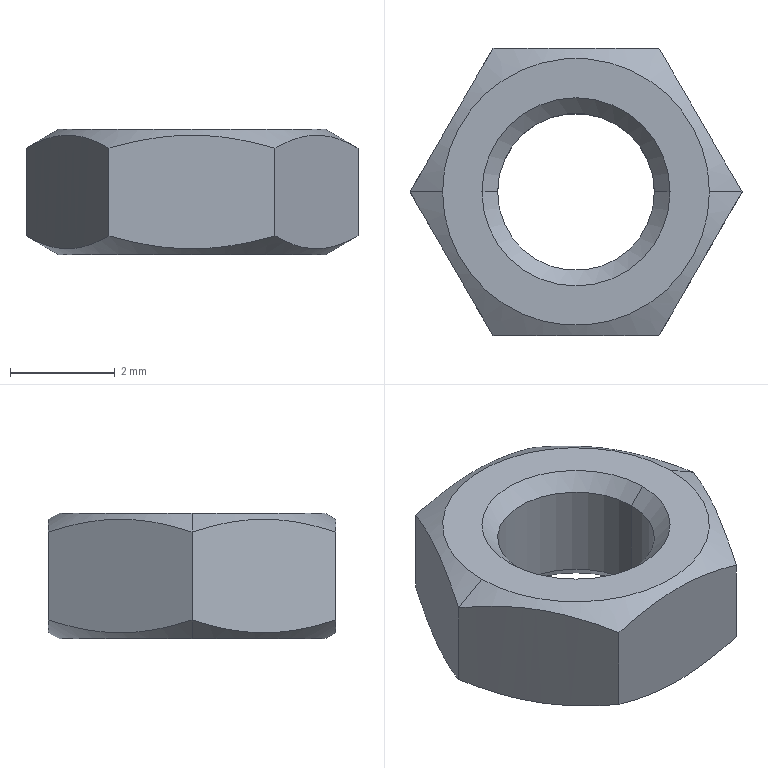Part | SolidWorks | features BaseBody 1 | 1 solid | 18 faces | box 6.351 x 5.5 x 2.4 mm | volume 43.705 mm3 | cone 8 | plane 8 | cylinder 2 | commonest cylinder face diameters 3 x2
STEP:
#1=CARTESIAN_POINT('',(-1.5,0.,2.1));
#2=VERTEX_POINT('',#1);
#3=CARTESIAN_POINT('',(-1.8,0.,2.4));
#4=VERTEX_POINT('',#3);
#5=CARTESIAN_POINT('',(-1.5,0.,2.1));
#6=DIRECTION('',(-0.7071,0.,0.7071));
#7=VECTOR('',#6,1000.);
#8=LINE('',#5,#7);
#9=EDGE_CURVE('',#2,#4,#8,.T.);
#10=ORIENTED_EDGE('',*,*,#9,.F.);
#11=CARTESIAN_POINT('',(1.5,0.,2.1));
#12=VERTEX_POINT('',#11);
#13=CARTESIAN_POINT('',(0.,0.,2.1));
#14=DIRECTION('',(0.,0.,1.));
#15=DIRECTION('',(1.,0.,0.));
#16=AXIS2_PLACEMENT_3D('',#13,#14,#15);
#17=CIRCLE('',#16,1.5);
#18=EDGE_CURVE('',#12,#2,#17,.T.);
#19=ORIENTED_EDGE('',*,*,#18,.F.);
#20=CARTESIAN_POINT('',(1.8,0.,2.4));
#21=VERTEX_POINT('',#20);
#22=CARTESIAN_POINT('',(1.5,0.,2.1));
#23=DIRECTION('',(0.7071,0.,0.7071));
#24=VECTOR('',#23,1000.);
#25=LINE('',#22,#24);
#26=EDGE_CURVE('',#12,#21,#25,.T.);
#27=ORIENTED_EDGE('',*,*,#26,.T.);
#28=CARTESIAN_POINT('',(0.,0.,2.4));
#29=DIRECTION('',(0.,0.,-1.));
#30=DIRECTION('',(1.,0.,0.));
#31=AXIS2_PLACEMENT_3D('',#28,#29,#30);
#32=CIRCLE('',#31,1.8);
#33=EDGE_CURVE('',#4,#21,#32,.T.);
#34=ORIENTED_EDGE('',*,*,#33,.F.);
#35=EDGE_LOOP('',(#10,#19,#27,#34));
#36=FACE_OUTER_BOUND('',#35,.T.);
#37=CARTESIAN_POINT('',(0.,0.,2.1));
#38=DIRECTION('',(0.,0.,1.));
#39=DIRECTION('',(1.,0.,0.));
#40=AXIS2_PLACEMENT_3D('',#37,#38,#39);
#41=CONICAL_SURFACE('',#40,1.5,0.7854);
#42=ADVANCED_FACE('',(#36),#41,.F.);
#43=CARTESIAN_POINT('',(1.5,0.,0.3));
#44=VERTEX_POINT('',#43);
#45=CARTESIAN_POINT('',(1.8,0.,0.));
#46=VERTEX_POINT('',#45);
#47=CARTESIAN_POINT('',(1.8,0.,0.));
#48=DIRECTION('',(0.7071,0.,-0.7071));
#49=VECTOR('',#48,1000.);
#50=LINE('',#47,#49);
#51=EDGE_CURVE('',#44,#46,#50,.T.);
#52=ORIENTED_EDGE('',*,*,#51,.F.);
#53=CARTESIAN_POINT('',(-1.5,0.,0.3));
#54=VERTEX_POINT('',#53);
#55=CARTESIAN_POINT('',(0.,0.,0.3));
#56=DIRECTION('',(0.,0.,-1.));
#57=DIRECTION('',(1.,0.,0.));
#58=AXIS2_PLACEMENT_3D('',#55,#56,#57);
#59=CIRCLE('',#58,1.5);
#60=EDGE_CURVE('',#54,#44,#59,.T.);
#61=ORIENTED_EDGE('',*,*,#60,.F.);
#62=CARTESIAN_POINT('',(-1.8,0.,0.));
#63=VERTEX_POINT('',#62);
#64=CARTESIAN_POINT('',(-1.8,0.,0.));
#65=DIRECTION('',(-0.7071,0.,-0.7071));
#66=VECTOR('',#65,1000.);
#67=LINE('',#64,#66);
#68=EDGE_CURVE('',#54,#63,#67,.T.);
#69=ORIENTED_EDGE('',*,*,#68,.T.);
#70=CARTESIAN_POINT('',(0.,0.,0.));
#71=DIRECTION('',(0.,0.,1.));
#72=DIRECTION('',(1.,0.,0.));
#73=AXIS2_PLACEMENT_3D('',#70,#71,#72);
#74=CIRCLE('',#73,1.8);
#75=EDGE_CURVE('',#46,#63,#74,.T.);
#76=ORIENTED_EDGE('',*,*,#75,.F.);
#77=EDGE_LOOP('',(#52,#61,#69,#76));
#78=FACE_OUTER_BOUND('',#77,.T.);
#79=CARTESIAN_POINT('',(0.,0.,0.));
#80=DIRECTION('',(0.,0.,-1.));
#81=DIRECTION('',(-1.,0.,0.));
#82=AXIS2_PLACEMENT_3D('',#79,#80,#81);
#83=CONICAL_SURFACE('',#82,1.8,0.7854);
#84=ADVANCED_FACE('',(#78),#83,.F.);
#85=CARTESIAN_POINT('',(-2.552,0.,2.4));
#86=VERTEX_POINT('',#85);
#87=CARTESIAN_POINT('',(-3.175,0.,2.04));
#88=VERTEX_POINT('',#87);
#89=CARTESIAN_POINT('',(-2.552,0.,2.4));
#90=DIRECTION('',(-0.866,0.,-0.5));
#91=VECTOR('',#90,1000.);
#92=LINE('',#89,#91);
#93=EDGE_CURVE('',#86,#88,#92,.T.);
#94=ORIENTED_EDGE('',*,*,#93,.F.);
#95=CARTESIAN_POINT('',(2.552,0.,2.4));
#96=VERTEX_POINT('',#95);
#97=CARTESIAN_POINT('',(0.,0.,2.4));
#98=DIRECTION('',(0.,0.,-1.));
#99=DIRECTION('',(-1.,0.,0.));
#100=AXIS2_PLACEMENT_3D('',#97,#98,#99);
#101=CIRCLE('',#100,2.552);
#102=EDGE_CURVE('',#86,#96,#101,.T.);
#103=ORIENTED_EDGE('',*,*,#102,.T.);
#104=CARTESIAN_POINT('',(3.175,0.,2.04));
#105=VERTEX_POINT('',#104);
#106=CARTESIAN_POINT('',(2.552,0.,2.4));
#107=DIRECTION('',(0.866,0.,-0.5));
#108=VECTOR('',#107,1000.);
#109=LINE('',#106,#108);
#110=EDGE_CURVE('',#96,#105,#109,.T.);
#111=ORIENTED_EDGE('',*,*,#110,.T.);
#112=CARTESIAN_POINT('',(1.588,2.75,2.04));
#113=VERTEX_POINT('',#112);
#114=CARTESIAN_POINT('',(3.175,0.,2.04));
#115=CARTESIAN_POINT('',(3.108,0.1168,2.079));
#116=CARTESIAN_POINT('',(3.042,0.2311,2.113));
#117=CARTESIAN_POINT('',(2.944,0.4004,2.158));
#118=CARTESIAN_POINT('',(2.912,0.4564,2.172));
#119=CARTESIAN_POINT('',(2.864,0.5402,2.191));
#120=CARTESIAN_POINT('',(2.848,0.568,2.197));
#121=CARTESIAN_POINT('',(2.816,0.6237,2.208));
#122=CARTESIAN_POINT('',(2.801,0.6497,2.214));
#123=CARTESIAN_POINT('',(2.647,0.9155,2.263));
#124=CARTESIAN_POINT('',(2.518,1.139,2.285));
#125=CARTESIAN_POINT('',(2.316,1.489,2.286));
#126=CARTESIAN_POINT('',(2.249,1.604,2.28));
#127=CARTESIAN_POINT('',(2.149,1.777,2.264));
#128=CARTESIAN_POINT('',(2.116,1.835,2.257));
#129=CARTESIAN_POINT('',(2.066,1.922,2.244));
#130=CARTESIAN_POINT('',(2.049,1.951,2.24));
#131=CARTESIAN_POINT('',(2.015,2.01,2.23));
#132=CARTESIAN_POINT('',(1.997,2.041,2.225));
#133=CARTESIAN_POINT('',(1.852,2.292,2.178));
#134=CARTESIAN_POINT('',(1.723,2.515,2.118));
#135=CARTESIAN_POINT('',(1.588,2.75,2.04));
#136=B_SPLINE_CURVE_WITH_KNOTS('',3,(#114,#115,#116,#117,#118,#119,#120,#121,#122,#123,#124,#125,#126,#127,#128,#129,#130,#131,#132,#133,#134,#135),.UNSPECIFIED.,.F.,.F.,(4,2,2,2,2,2,2,2,2,2,4),(0.,0.125,0.1875,0.2188,0.25,0.5,0.625,0.6875,0.7188,0.75,1.),.UNSPECIFIED.);
#137=EDGE_CURVE('',#105,#113,#136,.T.);
#138=ORIENTED_EDGE('',*,*,#137,.T.);
#139=CARTESIAN_POINT('',(-1.588,2.75,2.04));
#140=VERTEX_POINT('',#139);
#141=CARTESIAN_POINT('',(1.588,2.75,2.04));
#142=CARTESIAN_POINT('',(1.453,2.75,2.079));
#143=CARTESIAN_POINT('',(1.321,2.75,2.113));
#144=CARTESIAN_POINT('',(1.126,2.75,2.158));
#145=CARTESIAN_POINT('',(1.061,2.75,2.172));
#146=CARTESIAN_POINT('',(0.9645,2.75,2.191));
#147=CARTESIAN_POINT('',(0.9324,2.75,2.197));
#148=CARTESIAN_POINT('',(0.8682,2.75,2.208));
#149=CARTESIAN_POINT('',(0.8383,2.75,2.214));
#150=CARTESIAN_POINT('',(0.5302,2.75,2.263));
#151=CARTESIAN_POINT('',(0.2694,2.75,2.286));
#152=CARTESIAN_POINT('',(-0.1341,2.75,2.286));
#153=CARTESIAN_POINT('',(-0.2666,2.75,2.28));
#154=CARTESIAN_POINT('',(-0.4663,2.75,2.263));
#155=CARTESIAN_POINT('',(-0.5331,2.75,2.257));
#156=CARTESIAN_POINT('',(-0.6339,2.75,2.244));
#157=CARTESIAN_POINT('',(-0.6677,2.75,2.24));
#158=CARTESIAN_POINT('',(-0.7355,2.75,2.23));
#159=CARTESIAN_POINT('',(-0.7717,2.75,2.224));
#160=CARTESIAN_POINT('',(-1.06,2.75,2.178));
#161=CARTESIAN_POINT('',(-1.318,2.75,2.118));
#162=CARTESIAN_POINT('',(-1.588,2.75,2.04));
#163=B_SPLINE_CURVE_WITH_KNOTS('',3,(#141,#142,#143,#144,#145,#146,#147,#148,#149,#150,#151,#152,#153,#154,#155,#156,#157,#158,#159,#160,#161,#162),.UNSPECIFIED.,.F.,.F.,(4,2,2,2,2,2,2,2,2,2,4),(0.,0.125,0.1875,0.2187,0.25,0.5,0.625,0.6875,0.7187,0.75,1.),.UNSPECIFIED.);
#164=EDGE_CURVE('',#113,#140,#163,.T.);
#165=ORIENTED_EDGE('',*,*,#164,.T.);
#166=CARTESIAN_POINT('',(-1.588,2.75,2.04));
#167=CARTESIAN_POINT('',(-1.655,2.633,2.079));
#168=CARTESIAN_POINT('',(-1.721,2.519,2.113));
#169=CARTESIAN_POINT('',(-1.819,2.35,2.158));
#170=CARTESIAN_POINT('',(-1.851,2.294,2.172));
#171=CARTESIAN_POINT('',(-1.9,2.21,2.191));
#172=CARTESIAN_POINT('',(-1.916,2.182,2.197));
#173=CARTESIAN_POINT('',(-1.948,2.126,2.208));
#174=CARTESIAN_POINT('',(-1.963,2.1,2.214));
#175=CARTESIAN_POINT('',(-2.116,1.835,2.263));
#176=CARTESIAN_POINT('',(-2.245,1.611,2.285));
#177=CARTESIAN_POINT('',(-2.447,1.261,2.286));
#178=CARTESIAN_POINT('',(-2.514,1.146,2.28));
#179=CARTESIAN_POINT('',(-2.614,0.9728,2.264));
#180=CARTESIAN_POINT('',(-2.647,0.915,2.257));
#181=CARTESIAN_POINT('',(-2.697,0.8278,2.244));
#182=CARTESIAN_POINT('',(-2.714,0.7986,2.24));
#183=CARTESIAN_POINT('',(-2.748,0.7399,2.23));
#184=CARTESIAN_POINT('',(-2.766,0.7087,2.225));
#185=CARTESIAN_POINT('',(-2.911,0.4583,2.178));
#186=CARTESIAN_POINT('',(-3.04,0.2346,2.118));
#187=CARTESIAN_POINT('',(-3.175,0.,2.04));
#188=B_SPLINE_CURVE_WITH_KNOTS('',3,(#166,#167,#168,#169,#170,#171,#172,#173,#174,#175,#176,#177,#178,#179,#180,#181,#182,#183,#184,#185,#186,#187),.UNSPECIFIED.,.F.,.F.,(4,2,2,2,2,2,2,2,2,2,4),(0.,0.125,0.1875,0.2188,0.25,0.5,0.625,0.6875,0.7188,0.75,1.),.UNSPECIFIED.);
#189=EDGE_CURVE('',#140,#88,#188,.T.);
#190=ORIENTED_EDGE('',*,*,#189,.T.);
#191=EDGE_LOOP('',(#94,#103,#111,#138,#165,#190));
#192=FACE_OUTER_BOUND('',#191,.T.);
#193=CARTESIAN_POINT('',(0.,0.,2.4));
#194=DIRECTION('',(0.,0.,-1.));
#195=DIRECTION('',(1.,0.,0.));
#196=AXIS2_PLACEMENT_3D('',#193,#194,#195);
#197=CONICAL_SURFACE('',#196,2.552,1.047);
#198=ADVANCED_FACE('',(#192),#197,.T.);
#199=CARTESIAN_POINT('',(-2.552,0.,0.));
#200=VERTEX_POINT('',#199);
#201=CARTESIAN_POINT('',(-3.175,0.,0.36));
#202=VERTEX_POINT('',#201);
#203=CARTESIAN_POINT('',(-2.552,0.,0.));
#204=DIRECTION('',(-0.866,0.,0.5));
#205=VECTOR('',#204,1000.);
#206=LINE('',#203,#205);
#207=EDGE_CURVE('',#200,#202,#206,.T.);
#208=ORIENTED_EDGE('',*,*,#207,.F.);
#209=CARTESIAN_POINT('',(2.552,0.,0.));
#210=VERTEX_POINT('',#209);
#211=CARTESIAN_POINT('',(0.,0.,0.));
#212=DIRECTION('',(0.,0.,-1.));
#213=DIRECTION('',(-1.,0.,0.));
#214=AXIS2_PLACEMENT_3D('',#211,#212,#213);
#215=CIRCLE('',#214,2.552);
#216=EDGE_CURVE('',#210,#200,#215,.T.);
#217=ORIENTED_EDGE('',*,*,#216,.F.);
#218=CARTESIAN_POINT('',(3.175,0.,0.36));
#219=VERTEX_POINT('',#218);
#220=CARTESIAN_POINT('',(2.552,0.,0.));
#221=DIRECTION('',(0.866,0.,0.5));
#222=VECTOR('',#221,1000.);
#223=LINE('',#220,#222);
#224=EDGE_CURVE('',#210,#219,#223,.T.);
#225=ORIENTED_EDGE('',*,*,#224,.T.);
#226=CARTESIAN_POINT('',(1.588,-2.75,0.36));
#227=VERTEX_POINT('',#226);
#228=CARTESIAN_POINT('',(3.175,0.,0.36));
#229=CARTESIAN_POINT('',(3.108,-0.1168,0.3211));
#230=CARTESIAN_POINT('',(3.042,-0.2311,0.2867));
#231=CARTESIAN_POINT('',(2.944,-0.4004,0.2419));
#232=CARTESIAN_POINT('',(2.912,-0.4564,0.2281));
#233=CARTESIAN_POINT('',(2.864,-0.5402,0.2091));
#234=CARTESIAN_POINT('',(2.848,-0.568,0.2031));
#235=CARTESIAN_POINT('',(2.816,-0.6237,0.1915));
#236=CARTESIAN_POINT('',(2.801,-0.6497,0.1864));
#237=CARTESIAN_POINT('',(2.647,-0.9155,0.1367));
#238=CARTESIAN_POINT('',(2.518,-1.139,0.1146));
#239=CARTESIAN_POINT('',(2.316,-1.489,0.1143));
#240=CARTESIAN_POINT('',(2.249,-1.604,0.1198));
#241=CARTESIAN_POINT('',(2.149,-1.777,0.1363));
#242=CARTESIAN_POINT('',(2.116,-1.835,0.1432));
#243=CARTESIAN_POINT('',(2.066,-1.922,0.1556));
#244=CARTESIAN_POINT('',(2.049,-1.951,0.1601));
#245=CARTESIAN_POINT('',(2.015,-2.01,0.1697));
#246=CARTESIAN_POINT('',(1.997,-2.041,0.1753));
#247=CARTESIAN_POINT('',(1.852,-2.292,0.222));
#248=CARTESIAN_POINT('',(1.723,-2.515,0.2818));
#249=CARTESIAN_POINT('',(1.588,-2.75,0.36));
#250=B_SPLINE_CURVE_WITH_KNOTS('',3,(#228,#229,#230,#231,#232,#233,#234,#235,#236,#237,#238,#239,#240,#241,#242,#243,#244,#245,#246,#247,#248,#249),.UNSPECIFIED.,.F.,.F.,(4,2,2,2,2,2,2,2,2,2,4),(0.,0.125,0.1875,0.2187,0.25,0.5,0.625,0.6875,0.7188,0.75,1.),.UNSPECIFIED.);
#251=EDGE_CURVE('',#219,#227,#250,.T.);
#252=ORIENTED_EDGE('',*,*,#251,.T.);
#253=CARTESIAN_POINT('',(-1.588,-2.75,0.36));
#254=VERTEX_POINT('',#253);
#255=CARTESIAN_POINT('',(1.588,-2.75,0.36));
#256=CARTESIAN_POINT('',(1.453,-2.75,0.3211));
#257=CARTESIAN_POINT('',(1.321,-2.75,0.2867));
#258=CARTESIAN_POINT('',(1.126,-2.75,0.2419));
#259=CARTESIAN_POINT('',(1.061,-2.75,0.2281));
#260=CARTESIAN_POINT('',(0.9645,-2.75,0.2092));
#261=CARTESIAN_POINT('',(0.9324,-2.75,0.2031));
#262=CARTESIAN_POINT('',(0.8682,-2.75,0.1916));
#263=CARTESIAN_POINT('',(0.8383,-2.75,0.1865));
#264=CARTESIAN_POINT('',(0.5302,-2.75,0.1366));
#265=CARTESIAN_POINT('',(0.2694,-2.75,0.1144));
#266=CARTESIAN_POINT('',(-0.1341,-2.75,0.1144));
#267=CARTESIAN_POINT('',(-0.2666,-2.75,0.1199));
#268=CARTESIAN_POINT('',(-0.4663,-2.75,0.1365));
#269=CARTESIAN_POINT('',(-0.5331,-2.75,0.1435));
#270=CARTESIAN_POINT('',(-0.6339,-2.75,0.156));
#271=CARTESIAN_POINT('',(-0.6677,-2.75,0.1605));
#272=CARTESIAN_POINT('',(-0.7355,-2.75,0.1702));
#273=CARTESIAN_POINT('',(-0.7717,-2.75,0.1757));
#274=CARTESIAN_POINT('',(-1.06,-2.75,0.2224));
#275=CARTESIAN_POINT('',(-1.318,-2.75,0.2821));
#276=CARTESIAN_POINT('',(-1.588,-2.75,0.36));
#277=B_SPLINE_CURVE_WITH_KNOTS('',3,(#255,#256,#257,#258,#259,#260,#261,#262,#263,#264,#265,#266,#267,#268,#269,#270,#271,#272,#273,#274,#275,#276),.UNSPECIFIED.,.F.,.F.,(4,2,2,2,2,2,2,2,2,2,4),(0.,0.125,0.1875,0.2188,0.25,0.5,0.625,0.6875,0.7188,0.75,1.),.UNSPECIFIED.);
#278=EDGE_CURVE('',#227,#254,#277,.T.);
#279=ORIENTED_EDGE('',*,*,#278,.T.);
#280=CARTESIAN_POINT('',(-1.588,-2.75,0.36));
#281=CARTESIAN_POINT('',(-1.655,-2.633,0.3211));
#282=CARTESIAN_POINT('',(-1.721,-2.519,0.2867));
#283=CARTESIAN_POINT('',(-1.819,-2.35,0.2419));
#284=CARTESIAN_POINT('',(-1.851,-2.294,0.2281));
#285=CARTESIAN_POINT('',(-1.9,-2.21,0.2091));
#286=CARTESIAN_POINT('',(-1.916,-2.182,0.2031));
#287=CARTESIAN_POINT('',(-1.948,-2.126,0.1915));
#288=CARTESIAN_POINT('',(-1.963,-2.1,0.1864));
#289=CARTESIAN_POINT('',(-2.116,-1.835,0.1367));
#290=CARTESIAN_POINT('',(-2.245,-1.611,0.1146));
#291=CARTESIAN_POINT('',(-2.447,-1.261,0.1143));
#292=CARTESIAN_POINT('',(-2.514,-1.146,0.1198));
#293=CARTESIAN_POINT('',(-2.614,-0.9728,0.1363));
#294=CARTESIAN_POINT('',(-2.647,-0.915,0.1432));
#295=CARTESIAN_POINT('',(-2.697,-0.8278,0.1556));
#296=CARTESIAN_POINT('',(-2.714,-0.7986,0.1601));
#297=CARTESIAN_POINT('',(-2.748,-0.7399,0.1697));
#298=CARTESIAN_POINT('',(-2.766,-0.7087,0.1753));
#299=CARTESIAN_POINT('',(-2.911,-0.4583,0.222));
#300=CARTESIAN_POINT('',(-3.04,-0.2346,0.2818));
#301=CARTESIAN_POINT('',(-3.175,0.,0.36));
#302=B_SPLINE_CURVE_WITH_KNOTS('',3,(#280,#281,#282,#283,#284,#285,#286,#287,#288,#289,#290,#291,#292,#293,#294,#295,#296,#297,#298,#299,#300,#301),.UNSPECIFIED.,.F.,.F.,(4,2,2,2,2,2,2,2,2,2,4),(0.,0.125,0.1875,0.2187,0.25,0.5,0.625,0.6875,0.7187,0.75,1.),.UNSPECIFIED.);
#303=EDGE_CURVE('',#254,#202,#302,.T.);
#304=ORIENTED_EDGE('',*,*,#303,.T.);
#305=EDGE_LOOP('',(#208,#217,#225,#252,#279,#304));
#306=FACE_OUTER_BOUND('',#305,.T.);
#307=CARTESIAN_POINT('',(0.,0.,0.));
#308=DIRECTION('',(0.,0.,1.));
#309=DIRECTION('',(1.,0.,0.));
#310=AXIS2_PLACEMENT_3D('',#307,#308,#309);
#311=CONICAL_SURFACE('',#310,2.552,1.047);
#312=ADVANCED_FACE('',(#306),#311,.T.);
#313=CARTESIAN_POINT('',(1.5,0.,2.4));
#314=DIRECTION('',(0.,0.,-1.));
#315=VECTOR('',#314,1000.);
#316=LINE('',#313,#315);
#317=EDGE_CURVE('',#12,#44,#316,.T.);
#318=ORIENTED_EDGE('',*,*,#317,.F.);
#319=ORIENTED_EDGE('',*,*,#18,.T.);
#320=CARTESIAN_POINT('',(-1.5,0.,2.4));
#321=DIRECTION('',(0.,0.,-1.));
#322=VECTOR('',#321,1000.);
#323=LINE('',#320,#322);
#324=EDGE_CURVE('',#2,#54,#323,.T.);
#325=ORIENTED_EDGE('',*,*,#324,.T.);
#326=ORIENTED_EDGE('',*,*,#60,.T.);
#327=EDGE_LOOP('',(#318,#319,#325,#326));
#328=FACE_OUTER_BOUND('',#327,.T.);
#329=CARTESIAN_POINT('',(0.,0.,2.4));
#330=DIRECTION('',(0.,0.,-1.));
#331=DIRECTION('',(-1.,0.,0.));
#332=AXIS2_PLACEMENT_3D('',#329,#330,#331);
#333=CYLINDRICAL_SURFACE('',#332,1.5);
#334=ADVANCED_FACE('',(#328),#333,.F.);
#335=CARTESIAN_POINT('',(0.,0.,0.));
#336=DIRECTION('',(0.,0.,1.));
#337=DIRECTION('',(1.,0.,0.));
#338=AXIS2_PLACEMENT_3D('',#335,#336,#337);
#339=CIRCLE('',#338,1.8);
#340=EDGE_CURVE('',#63,#46,#339,.T.);
#341=ORIENTED_EDGE('',*,*,#340,.T.);
#342=ORIENTED_EDGE('',*,*,#75,.T.);
#343=EDGE_LOOP('',(#341,#342));
#344=FACE_BOUND('',#343,.T.);
#345=ORIENTED_EDGE('',*,*,#216,.T.);
#346=CARTESIAN_POINT('',(0.,0.,0.));
#347=DIRECTION('',(0.,0.,-1.));
#348=DIRECTION('',(-1.,0.,0.));
#349=AXIS2_PLACEMENT_3D('',#346,#347,#348);
#350=CIRCLE('',#349,2.552);
#351=EDGE_CURVE('',#200,#210,#350,.T.);
#352=ORIENTED_EDGE('',*,*,#351,.T.);
#353=EDGE_LOOP('',(#345,#352));
#354=FACE_OUTER_BOUND('',#353,.T.);
#355=CARTESIAN_POINT('',(0.,0.,0.));
#356=DIRECTION('',(0.,0.,1.));
#357=DIRECTION('',(1.,0.,0.));
#358=AXIS2_PLACEMENT_3D('',#355,#356,#357);
#359=PLANE('',#358);
#360=ADVANCED_FACE('',(#344,#354),#359,.F.);
#361=CARTESIAN_POINT('',(0.,0.,2.4));
#362=DIRECTION('',(0.,0.,-1.));
#363=DIRECTION('',(1.,0.,0.));
#364=AXIS2_PLACEMENT_3D('',#361,#362,#363);
#365=CIRCLE('',#364,1.8);
#366=EDGE_CURVE('',#21,#4,#365,.T.);
#367=ORIENTED_EDGE('',*,*,#366,.T.);
#368=ORIENTED_EDGE('',*,*,#33,.T.);
#369=EDGE_LOOP('',(#367,#368));
#370=FACE_BOUND('',#369,.T.);
#371=CARTESIAN_POINT('',(0.,0.,2.4));
#372=DIRECTION('',(0.,0.,-1.));
#373=DIRECTION('',(-1.,0.,0.));
#374=AXIS2_PLACEMENT_3D('',#371,#372,#373);
#375=CIRCLE('',#374,2.552);
#376=EDGE_CURVE('',#96,#86,#375,.T.);
#377=ORIENTED_EDGE('',*,*,#376,.F.);
#378=ORIENTED_EDGE('',*,*,#102,.F.);
#379=EDGE_LOOP('',(#377,#378));
#380=FACE_OUTER_BOUND('',#379,.T.);
#381=CARTESIAN_POINT('',(0.,0.,2.4));
#382=DIRECTION('',(0.,0.,1.));
#383=DIRECTION('',(1.,0.,0.));
#384=AXIS2_PLACEMENT_3D('',#381,#382,#383);
#385=PLANE('',#384);
#386=ADVANCED_FACE('',(#370,#380),#385,.T.);
#387=ORIENTED_EDGE('',*,*,#164,.F.);
#388=CARTESIAN_POINT('',(1.588,2.75,0.36));
#389=VERTEX_POINT('',#388);
#390=CARTESIAN_POINT('',(1.588,2.75,2.4));
#391=DIRECTION('',(0.,0.,-1.));
#392=VECTOR('',#391,1000.);
#393=LINE('',#390,#392);
#394=EDGE_CURVE('',#113,#389,#393,.T.);
#395=ORIENTED_EDGE('',*,*,#394,.T.);
#396=CARTESIAN_POINT('',(-1.588,2.75,0.36));
#397=VERTEX_POINT('',#396);
#398=CARTESIAN_POINT('',(-1.588,2.75,0.36));
#399=CARTESIAN_POINT('',(-1.453,2.75,0.3211));
#400=CARTESIAN_POINT('',(-1.321,2.75,0.2867));
#401=CARTESIAN_POINT('',(-1.126,2.75,0.2419));
#402=CARTESIAN_POINT('',(-1.061,2.75,0.2281));
#403=CARTESIAN_POINT('',(-0.9645,2.75,0.2092));
#404=CARTESIAN_POINT('',(-0.9324,2.75,0.2031));
#405=CARTESIAN_POINT('',(-0.8682,2.75,0.1916));
#406=CARTESIAN_POINT('',(-0.8383,2.75,0.1865));
#407=CARTESIAN_POINT('',(-0.5302,2.75,0.1366));
#408=CARTESIAN_POINT('',(-0.2694,2.75,0.1144));
#409=CARTESIAN_POINT('',(0.1341,2.75,0.1144));
#410=CARTESIAN_POINT('',(0.2666,2.75,0.1199));
#411=CARTESIAN_POINT('',(0.4663,2.75,0.1365));
#412=CARTESIAN_POINT('',(0.5331,2.75,0.1435));
#413=CARTESIAN_POINT('',(0.6339,2.75,0.156));
#414=CARTESIAN_POINT('',(0.6677,2.75,0.1605));
#415=CARTESIAN_POINT('',(0.7355,2.75,0.1702));
#416=CARTESIAN_POINT('',(0.7717,2.75,0.1757));
#417=CARTESIAN_POINT('',(1.06,2.75,0.2224));
#418=CARTESIAN_POINT('',(1.318,2.75,0.2821));
#419=CARTESIAN_POINT('',(1.588,2.75,0.36));
#420=B_SPLINE_CURVE_WITH_KNOTS('',3,(#398,#399,#400,#401,#402,#403,#404,#405,#406,#407,#408,#409,#410,#411,#412,#413,#414,#415,#416,#417,#418,#419),.UNSPECIFIED.,.F.,.F.,(4,2,2,2,2,2,2,2,2,2,4),(0.,0.125,0.1875,0.2187,0.25,0.5,0.625,0.6875,0.7187,0.75,1.),.UNSPECIFIED.);
#421=EDGE_CURVE('',#397,#389,#420,.T.);
#422=ORIENTED_EDGE('',*,*,#421,.F.);
#423=CARTESIAN_POINT('',(-1.588,2.75,2.4));
#424=DIRECTION('',(0.,0.,-1.));
#425=VECTOR('',#424,1000.);
#426=LINE('',#423,#425);
#427=EDGE_CURVE('',#140,#397,#426,.T.);
#428=ORIENTED_EDGE('',*,*,#427,.F.);
#429=EDGE_LOOP('',(#387,#395,#422,#428));
#430=FACE_OUTER_BOUND('',#429,.T.);
#431=CARTESIAN_POINT('',(1.588,2.75,2.4));
#432=DIRECTION('',(0.,-1.,0.));
#433=DIRECTION('',(0.,0.,-1.));
#434=AXIS2_PLACEMENT_3D('',#431,#432,#433);
#435=PLANE('',#434);
#436=ADVANCED_FACE('',(#430),#435,.F.);
#437=ORIENTED_EDGE('',*,*,#137,.F.);
#438=CARTESIAN_POINT('',(3.175,0.,2.4));
#439=DIRECTION('',(0.,0.,-1.));
#440=VECTOR('',#439,1000.);
#441=LINE('',#438,#440);
#442=EDGE_CURVE('',#105,#219,#441,.T.);
#443=ORIENTED_EDGE('',*,*,#442,.T.);
#444=CARTESIAN_POINT('',(1.588,2.75,0.36));
#445=CARTESIAN_POINT('',(1.655,2.633,0.3211));
#446=CARTESIAN_POINT('',(1.721,2.519,0.2867));
#447=CARTESIAN_POINT('',(1.819,2.35,0.2419));
#448=CARTESIAN_POINT('',(1.851,2.294,0.2281));
#449=CARTESIAN_POINT('',(1.9,2.21,0.2091));
#450=CARTESIAN_POINT('',(1.916,2.182,0.2031));
#451=CARTESIAN_POINT('',(1.948,2.126,0.1915));
#452=CARTESIAN_POINT('',(1.963,2.1,0.1864));
#453=CARTESIAN_POINT('',(2.116,1.835,0.1367));
#454=CARTESIAN_POINT('',(2.245,1.611,0.1146));
#455=CARTESIAN_POINT('',(2.447,1.261,0.1143));
#456=CARTESIAN_POINT('',(2.514,1.146,0.1198));
#457=CARTESIAN_POINT('',(2.614,0.9728,0.1363));
#458=CARTESIAN_POINT('',(2.647,0.915,0.1432));
#459=CARTESIAN_POINT('',(2.697,0.8278,0.1556));
#460=CARTESIAN_POINT('',(2.714,0.7986,0.1601));
#461=CARTESIAN_POINT('',(2.748,0.7399,0.1697));
#462=CARTESIAN_POINT('',(2.766,0.7087,0.1753));
#463=CARTESIAN_POINT('',(2.911,0.4583,0.222));
#464=CARTESIAN_POINT('',(3.04,0.2346,0.2818));
#465=CARTESIAN_POINT('',(3.175,0.,0.36));
#466=B_SPLINE_CURVE_WITH_KNOTS('',3,(#444,#445,#446,#447,#448,#449,#450,#451,#452,#453,#454,#455,#456,#457,#458,#459,#460,#461,#462,#463,#464,#465),.UNSPECIFIED.,.F.,.F.,(4,2,2,2,2,2,2,2,2,2,4),(0.,0.125,0.1875,0.2188,0.25,0.5,0.625,0.6875,0.7188,0.75,1.),.UNSPECIFIED.);
#467=EDGE_CURVE('',#389,#219,#466,.T.);
#468=ORIENTED_EDGE('',*,*,#467,.F.);
#469=ORIENTED_EDGE('',*,*,#394,.F.);
#470=EDGE_LOOP('',(#437,#443,#468,#469));
#471=FACE_OUTER_BOUND('',#470,.T.);
#472=CARTESIAN_POINT('',(3.175,0.,2.4));
#473=DIRECTION('',(-0.866,-0.5,0.));
#474=DIRECTION('',(-0.5,0.866,0.));
#475=AXIS2_PLACEMENT_3D('',#472,#473,#474);
#476=PLANE('',#475);
#477=ADVANCED_FACE('',(#471),#476,.F.);
#478=CARTESIAN_POINT('',(1.588,-2.75,2.04));
#479=VERTEX_POINT('',#478);
#480=CARTESIAN_POINT('',(1.588,-2.75,2.04));
#481=CARTESIAN_POINT('',(1.655,-2.633,2.079));
#482=CARTESIAN_POINT('',(1.721,-2.519,2.113));
#483=CARTESIAN_POINT('',(1.819,-2.35,2.158));
#484=CARTESIAN_POINT('',(1.851,-2.294,2.172));
#485=CARTESIAN_POINT('',(1.9,-2.21,2.191));
#486=CARTESIAN_POINT('',(1.916,-2.182,2.197));
#487=CARTESIAN_POINT('',(1.948,-2.126,2.208));
#488=CARTESIAN_POINT('',(1.963,-2.1,2.214));
#489=CARTESIAN_POINT('',(2.116,-1.835,2.263));
#490=CARTESIAN_POINT('',(2.245,-1.611,2.285));
#491=CARTESIAN_POINT('',(2.447,-1.261,2.286));
#492=CARTESIAN_POINT('',(2.514,-1.146,2.28));
#493=CARTESIAN_POINT('',(2.614,-0.9728,2.264));
#494=CARTESIAN_POINT('',(2.647,-0.915,2.257));
#495=CARTESIAN_POINT('',(2.697,-0.8278,2.244));
#496=CARTESIAN_POINT('',(2.714,-0.7986,2.24));
#497=CARTESIAN_POINT('',(2.748,-0.7399,2.23));
#498=CARTESIAN_POINT('',(2.766,-0.7087,2.225));
#499=CARTESIAN_POINT('',(2.911,-0.4583,2.178));
#500=CARTESIAN_POINT('',(3.04,-0.2346,2.118));
#501=CARTESIAN_POINT('',(3.175,0.,2.04));
#502=B_SPLINE_CURVE_WITH_KNOTS('',3,(#480,#481,#482,#483,#484,#485,#486,#487,#488,#489,#490,#491,#492,#493,#494,#495,#496,#497,#498,#499,#500,#501),.UNSPECIFIED.,.F.,.F.,(4,2,2,2,2,2,2,2,2,2,4),(0.,0.125,0.1875,0.2187,0.25,0.5,0.625,0.6875,0.7187,0.75,1.),.UNSPECIFIED.);
#503=EDGE_CURVE('',#479,#105,#502,.T.);
#504=ORIENTED_EDGE('',*,*,#503,.F.);
#505=CARTESIAN_POINT('',(1.588,-2.75,2.4));
#506=DIRECTION('',(0.,0.,-1.));
#507=VECTOR('',#506,1000.);
#508=LINE('',#505,#507);
#509=EDGE_CURVE('',#479,#227,#508,.T.);
#510=ORIENTED_EDGE('',*,*,#509,.T.);
#511=ORIENTED_EDGE('',*,*,#251,.F.);
#512=ORIENTED_EDGE('',*,*,#442,.F.);
#513=EDGE_LOOP('',(#504,#510,#511,#512));
#514=FACE_OUTER_BOUND('',#513,.T.);
#515=CARTESIAN_POINT('',(1.588,-2.75,2.4));
#516=DIRECTION('',(-0.866,0.5,0.));
#517=DIRECTION('',(0.,0.,1.));
#518=AXIS2_PLACEMENT_3D('',#515,#516,#517);
#519=PLANE('',#518);
#520=ADVANCED_FACE('',(#514),#519,.F.);
#521=CARTESIAN_POINT('',(-1.588,-2.75,2.04));
#522=VERTEX_POINT('',#521);
#523=CARTESIAN_POINT('',(-1.588,-2.75,2.04));
#524=CARTESIAN_POINT('',(-1.453,-2.75,2.079));
#525=CARTESIAN_POINT('',(-1.321,-2.75,2.113));
#526=CARTESIAN_POINT('',(-1.126,-2.75,2.158));
#527=CARTESIAN_POINT('',(-1.061,-2.75,2.172));
#528=CARTESIAN_POINT('',(-0.9645,-2.75,2.191));
#529=CARTESIAN_POINT('',(-0.9324,-2.75,2.197));
#530=CARTESIAN_POINT('',(-0.8682,-2.75,2.208));
#531=CARTESIAN_POINT('',(-0.8383,-2.75,2.214));
#532=CARTESIAN_POINT('',(-0.5302,-2.75,2.263));
#533=CARTESIAN_POINT('',(-0.2694,-2.75,2.286));
#534=CARTESIAN_POINT('',(0.1341,-2.75,2.286));
#535=CARTESIAN_POINT('',(0.2666,-2.75,2.28));
#536=CARTESIAN_POINT('',(0.4663,-2.75,2.263));
#537=CARTESIAN_POINT('',(0.5331,-2.75,2.257));
#538=CARTESIAN_POINT('',(0.6339,-2.75,2.244));
#539=CARTESIAN_POINT('',(0.6677,-2.75,2.24));
#540=CARTESIAN_POINT('',(0.7355,-2.75,2.23));
#541=CARTESIAN_POINT('',(0.7717,-2.75,2.224));
#542=CARTESIAN_POINT('',(1.06,-2.75,2.178));
#543=CARTESIAN_POINT('',(1.318,-2.75,2.118));
#544=CARTESIAN_POINT('',(1.588,-2.75,2.04));
#545=B_SPLINE_CURVE_WITH_KNOTS('',3,(#523,#524,#525,#526,#527,#528,#529,#530,#531,#532,#533,#534,#535,#536,#537,#538,#539,#540,#541,#542,#543,#544),.UNSPECIFIED.,.F.,.F.,(4,2,2,2,2,2,2,2,2,2,4),(0.,0.125,0.1875,0.2187,0.25,0.5,0.625,0.6875,0.7187,0.75,1.),.UNSPECIFIED.);
#546=EDGE_CURVE('',#522,#479,#545,.T.);
#547=ORIENTED_EDGE('',*,*,#546,.F.);
#548=CARTESIAN_POINT('',(-1.588,-2.75,2.4));
#549=DIRECTION('',(0.,0.,-1.));
#550=VECTOR('',#549,1000.);
#551=LINE('',#548,#550);
#552=EDGE_CURVE('',#522,#254,#551,.T.);
#553=ORIENTED_EDGE('',*,*,#552,.T.);
#554=ORIENTED_EDGE('',*,*,#278,.F.);
#555=ORIENTED_EDGE('',*,*,#509,.F.);
#556=EDGE_LOOP('',(#547,#553,#554,#555));
#557=FACE_OUTER_BOUND('',#556,.T.);
#558=CARTESIAN_POINT('',(-1.588,-2.75,2.4));
#559=DIRECTION('',(0.,1.,0.));
#560=DIRECTION('',(1.,0.,0.));
#561=AXIS2_PLACEMENT_3D('',#558,#559,#560);
#562=PLANE('',#561);
#563=ADVANCED_FACE('',(#557),#562,.F.);
#564=CARTESIAN_POINT('',(-3.175,0.,2.04));
#565=CARTESIAN_POINT('',(-3.108,-0.1168,2.079));
#566=CARTESIAN_POINT('',(-3.042,-0.2311,2.113));
#567=CARTESIAN_POINT('',(-2.944,-0.4004,2.158));
#568=CARTESIAN_POINT('',(-2.912,-0.4564,2.172));
#569=CARTESIAN_POINT('',(-2.864,-0.5402,2.191));
#570=CARTESIAN_POINT('',(-2.848,-0.568,2.197));
#571=CARTESIAN_POINT('',(-2.816,-0.6237,2.208));
#572=CARTESIAN_POINT('',(-2.801,-0.6497,2.214));
#573=CARTESIAN_POINT('',(-2.647,-0.9155,2.263));
#574=CARTESIAN_POINT('',(-2.518,-1.139,2.285));
#575=CARTESIAN_POINT('',(-2.316,-1.489,2.286));
#576=CARTESIAN_POINT('',(-2.249,-1.604,2.28));
#577=CARTESIAN_POINT('',(-2.149,-1.777,2.264));
#578=CARTESIAN_POINT('',(-2.116,-1.835,2.257));
#579=CARTESIAN_POINT('',(-2.066,-1.922,2.244));
#580=CARTESIAN_POINT('',(-2.049,-1.951,2.24));
#581=CARTESIAN_POINT('',(-2.015,-2.01,2.23));
#582=CARTESIAN_POINT('',(-1.997,-2.041,2.225));
#583=CARTESIAN_POINT('',(-1.852,-2.292,2.178));
#584=CARTESIAN_POINT('',(-1.723,-2.515,2.118));
#585=CARTESIAN_POINT('',(-1.588,-2.75,2.04));
#586=B_SPLINE_CURVE_WITH_KNOTS('',3,(#564,#565,#566,#567,#568,#569,#570,#571,#572,#573,#574,#575,#576,#577,#578,#579,#580,#581,#582,#583,#584,#585),.UNSPECIFIED.,.F.,.F.,(4,2,2,2,2,2,2,2,2,2,4),(0.,0.125,0.1875,0.2187,0.25,0.5,0.625,0.6875,0.7188,0.75,1.),.UNSPECIFIED.);
#587=EDGE_CURVE('',#88,#522,#586,.T.);
#588=ORIENTED_EDGE('',*,*,#587,.F.);
#589=CARTESIAN_POINT('',(-3.175,0.,2.4));
#590=DIRECTION('',(0.,0.,-1.));
#591=VECTOR('',#590,1000.);
#592=LINE('',#589,#591);
#593=EDGE_CURVE('',#88,#202,#592,.T.);
#594=ORIENTED_EDGE('',*,*,#593,.T.);
#595=ORIENTED_EDGE('',*,*,#303,.F.);
#596=ORIENTED_EDGE('',*,*,#552,.F.);
#597=EDGE_LOOP('',(#588,#594,#595,#596));
#598=FACE_OUTER_BOUND('',#597,.T.);
#599=CARTESIAN_POINT('',(-3.175,0.,2.4));
#600=DIRECTION('',(0.866,0.5,0.));
#601=DIRECTION('',(0.,0.,-1.));
#602=AXIS2_PLACEMENT_3D('',#599,#600,#601);
#603=PLANE('',#602);
#604=ADVANCED_FACE('',(#598),#603,.F.);
#605=ORIENTED_EDGE('',*,*,#189,.F.);
#606=ORIENTED_EDGE('',*,*,#427,.T.);
#607=CARTESIAN_POINT('',(-3.175,0.,0.36));
#608=CARTESIAN_POINT('',(-3.108,0.1168,0.3211));
#609=CARTESIAN_POINT('',(-3.042,0.2311,0.2867));
#610=CARTESIAN_POINT('',(-2.944,0.4004,0.2419));
#611=CARTESIAN_POINT('',(-2.912,0.4564,0.2281));
#612=CARTESIAN_POINT('',(-2.864,0.5402,0.2091));
#613=CARTESIAN_POINT('',(-2.848,0.568,0.2031));
#614=CARTESIAN_POINT('',(-2.816,0.6237,0.1915));
#615=CARTESIAN_POINT('',(-2.801,0.6497,0.1864));
#616=CARTESIAN_POINT('',(-2.647,0.9155,0.1367));
#617=CARTESIAN_POINT('',(-2.518,1.139,0.1146));
#618=CARTESIAN_POINT('',(-2.316,1.489,0.1143));
#619=CARTESIAN_POINT('',(-2.249,1.604,0.1198));
#620=CARTESIAN_POINT('',(-2.149,1.777,0.1363));
#621=CARTESIAN_POINT('',(-2.116,1.835,0.1432));
#622=CARTESIAN_POINT('',(-2.066,1.922,0.1556));
#623=CARTESIAN_POINT('',(-2.049,1.951,0.1601));
#624=CARTESIAN_POINT('',(-2.015,2.01,0.1697));
#625=CARTESIAN_POINT('',(-1.997,2.041,0.1753));
#626=CARTESIAN_POINT('',(-1.852,2.292,0.222));
#627=CARTESIAN_POINT('',(-1.723,2.515,0.2818));
#628=CARTESIAN_POINT('',(-1.588,2.75,0.36));
#629=B_SPLINE_CURVE_WITH_KNOTS('',3,(#607,#608,#609,#610,#611,#612,#613,#614,#615,#616,#617,#618,#619,#620,#621,#622,#623,#624,#625,#626,#627,#628),.UNSPECIFIED.,.F.,.F.,(4,2,2,2,2,2,2,2,2,2,4),(0.,0.125,0.1875,0.2188,0.25,0.5,0.625,0.6875,0.7188,0.75,1.),.UNSPECIFIED.);
#630=EDGE_CURVE('',#202,#397,#629,.T.);
#631=ORIENTED_EDGE('',*,*,#630,.F.);
#632=ORIENTED_EDGE('',*,*,#593,.F.);
#633=EDGE_LOOP('',(#605,#606,#631,#632));
#634=FACE_OUTER_BOUND('',#633,.T.);
#635=CARTESIAN_POINT('',(-1.588,2.75,2.4));
#636=DIRECTION('',(0.866,-0.5,0.));
#637=DIRECTION('',(0.,0.,-1.));
#638=AXIS2_PLACEMENT_3D('',#635,#636,#637);
#639=PLANE('',#638);
#640=ADVANCED_FACE('',(#634),#639,.F.);
#641=CARTESIAN_POINT('',(0.,0.,2.1));
#642=DIRECTION('',(0.,0.,1.));
#643=DIRECTION('',(1.,0.,0.));
#644=AXIS2_PLACEMENT_3D('',#641,#642,#643);
#645=CIRCLE('',#644,1.5);
#646=EDGE_CURVE('',#2,#12,#645,.T.);
#647=ORIENTED_EDGE('',*,*,#646,.T.);
#648=ORIENTED_EDGE('',*,*,#317,.T.);
#649=CARTESIAN_POINT('',(0.,0.,0.3));
#650=DIRECTION('',(0.,0.,-1.));
#651=DIRECTION('',(1.,0.,0.));
#652=AXIS2_PLACEMENT_3D('',#649,#650,#651);
#653=CIRCLE('',#652,1.5);
#654=EDGE_CURVE('',#44,#54,#653,.T.);
#655=ORIENTED_EDGE('',*,*,#654,.T.);
#656=ORIENTED_EDGE('',*,*,#324,.F.);
#657=EDGE_LOOP('',(#647,#648,#655,#656));
#658=FACE_OUTER_BOUND('',#657,.T.);
#659=CARTESIAN_POINT('',(0.,0.,2.4));
#660=DIRECTION('',(0.,0.,-1.));
#661=DIRECTION('',(-1.,0.,0.));
#662=AXIS2_PLACEMENT_3D('',#659,#660,#661);
#663=CYLINDRICAL_SURFACE('',#662,1.5);
#664=ADVANCED_FACE('',(#658),#663,.F.);
#665=ORIENTED_EDGE('',*,*,#351,.F.);
#666=ORIENTED_EDGE('',*,*,#207,.T.);
#667=ORIENTED_EDGE('',*,*,#630,.T.);
#668=ORIENTED_EDGE('',*,*,#421,.T.);
#669=ORIENTED_EDGE('',*,*,#467,.T.);
#670=ORIENTED_EDGE('',*,*,#224,.F.);
#671=EDGE_LOOP('',(#665,#666,#667,#668,#669,#670));
#672=FACE_OUTER_BOUND('',#671,.T.);
#673=CARTESIAN_POINT('',(0.,0.,0.));
#674=DIRECTION('',(0.,0.,1.));
#675=DIRECTION('',(1.,0.,0.));
#676=AXIS2_PLACEMENT_3D('',#673,#674,#675);
#677=CONICAL_SURFACE('',#676,2.552,1.047);
#678=ADVANCED_FACE('',(#672),#677,.T.);
#679=ORIENTED_EDGE('',*,*,#376,.T.);
#680=ORIENTED_EDGE('',*,*,#93,.T.);
#681=ORIENTED_EDGE('',*,*,#587,.T.);
#682=ORIENTED_EDGE('',*,*,#546,.T.);
#683=ORIENTED_EDGE('',*,*,#503,.T.);
#684=ORIENTED_EDGE('',*,*,#110,.F.);
#685=EDGE_LOOP('',(#679,#680,#681,#682,#683,#684));
#686=FACE_OUTER_BOUND('',#685,.T.);
#687=CARTESIAN_POINT('',(0.,0.,2.4));
#688=DIRECTION('',(0.,0.,-1.));
#689=DIRECTION('',(1.,0.,0.));
#690=AXIS2_PLACEMENT_3D('',#687,#688,#689);
#691=CONICAL_SURFACE('',#690,2.552,1.047);
#692=ADVANCED_FACE('',(#686),#691,.T.);
#693=ORIENTED_EDGE('',*,*,#654,.F.);
#694=ORIENTED_EDGE('',*,*,#51,.T.);
#695=ORIENTED_EDGE('',*,*,#340,.F.);
#696=ORIENTED_EDGE('',*,*,#68,.F.);
#697=EDGE_LOOP('',(#693,#694,#695,#696));
#698=FACE_OUTER_BOUND('',#697,.T.);
#699=CARTESIAN_POINT('',(0.,0.,0.));
#700=DIRECTION('',(0.,0.,-1.));
#701=DIRECTION('',(-1.,0.,0.));
#702=AXIS2_PLACEMENT_3D('',#699,#700,#701);
#703=CONICAL_SURFACE('',#702,1.8,0.7854);
#704=ADVANCED_FACE('',(#698),#703,.F.);
#705=ORIENTED_EDGE('',*,*,#646,.F.);
#706=ORIENTED_EDGE('',*,*,#9,.T.);
#707=ORIENTED_EDGE('',*,*,#366,.F.);
#708=ORIENTED_EDGE('',*,*,#26,.F.);
#709=EDGE_LOOP('',(#705,#706,#707,#708));
#710=FACE_OUTER_BOUND('',#709,.T.);
#711=CARTESIAN_POINT('',(0.,0.,2.1));
#712=DIRECTION('',(0.,0.,1.));
#713=DIRECTION('',(1.,0.,0.));
#714=AXIS2_PLACEMENT_3D('',#711,#712,#713);
#715=CONICAL_SURFACE('',#714,1.5,0.7854);
#716=ADVANCED_FACE('',(#710),#715,.F.);
#717=CLOSED_SHELL('',(#42,#84,#198,#312,#334,#360,#386,#436,#477,#520,#563,#604,#640,#664,#678,#692,#704,#716));
#718=MANIFOLD_SOLID_BREP('',#717);
#719=CARTESIAN_POINT('',(0.,0.,0.));
#720=DIRECTION('',(0.,0.,1.));
#721=DIRECTION('',(1.,0.,0.));
#722=AXIS2_PLACEMENT_3D('',#719,#720,#721);
#723=(LENGTH_UNIT()NAMED_UNIT(*)SI_UNIT(.MILLI.,.METRE.));
#724=UNCERTAINTY_MEASURE_WITH_UNIT(LENGTH_MEASURE(0.00001),#723,'','');
#725=(NAMED_UNIT(*)PLANE_ANGLE_UNIT()SI_UNIT($,.RADIAN.));
#726=(NAMED_UNIT(*)SI_UNIT($,.STERADIAN.)SOLID_ANGLE_UNIT());
#727=(GEOMETRIC_REPRESENTATION_CONTEXT(3)GLOBAL_UNCERTAINTY_ASSIGNED_CONTEXT((#724))GLOBAL_UNIT_ASSIGNED_CONTEXT((#723,#725,#726))REPRESENTATION_CONTEXT('',''));
#728=ADVANCED_BREP_SHAPE_REPRESENTATION('',(#718,#722),#727);